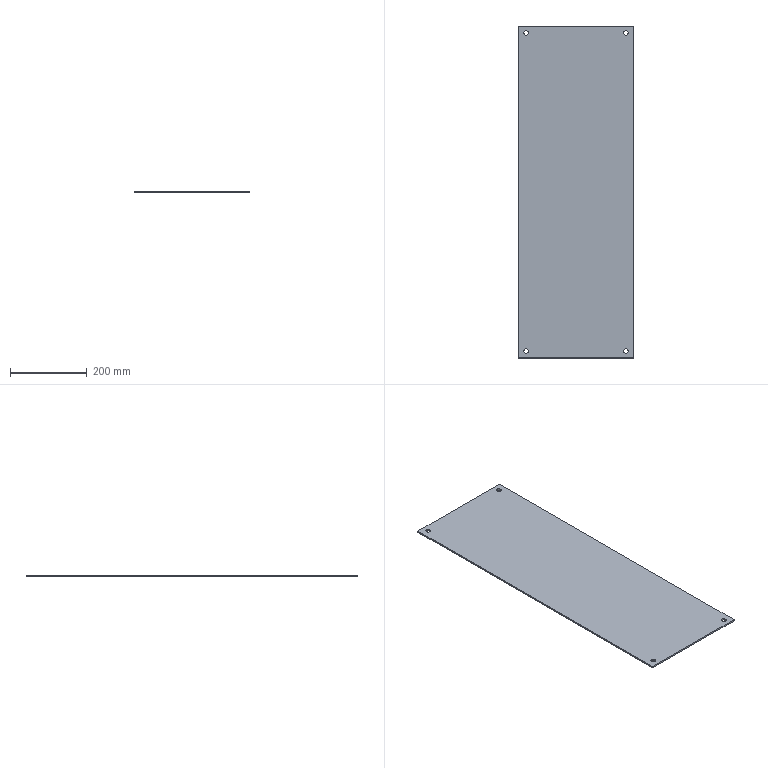Part | STEP file | 01 End cover plate | 1 solid | 14 faces | box 300 x 866 x 4 mm | volume 1037390 mm3 | cylinder 8 | plane 6 | commonest cylinder face diameters 12 x8
STEP:
#1=CARTESIAN_POINT('',(0.,0.,0.));
#2=DIRECTION('',(0.,0.,1.));
#3=DIRECTION('',(1.,0.,0.));
#4=AXIS2_PLACEMENT_3D('',#1,#2,#3);
#5=CARTESIAN_POINT('',(14.,-18.,4.));
#6=VERTEX_POINT('',#5);
#7=CARTESIAN_POINT('',(14.,-18.,0.));
#8=VERTEX_POINT('',#7);
#9=CARTESIAN_POINT('',(14.,-18.,4.));
#10=DIRECTION('',(0.,0.,-1.));
#11=VECTOR('',#10,1.);
#12=LINE('',#9,#11);
#13=CARTESIAN_POINT('',(20.,-18.,4.));
#14=DIRECTION('',(0.,0.,-1.));
#15=DIRECTION('',(-1.,0.,0.));
#16=AXIS2_PLACEMENT_3D('',#13,#14,#15);
#17=CYLINDRICAL_SURFACE('',#16,6.);
#18=CARTESIAN_POINT('',(6.283,0.));
#19=DIRECTION('',(0.,1.));
#20=VECTOR('',#19,1.);
#21=LINE('',#18,#20);
#22=(GEOMETRIC_REPRESENTATION_CONTEXT(2)PARAMETRIC_REPRESENTATION_CONTEXT()REPRESENTATION_CONTEXT('',''));
#23=DEFINITIONAL_REPRESENTATION('',(#21),#22);
#24=PCURVE('',#17,#23);
#25=CARTESIAN_POINT('',(20.,-18.,4.));
#26=DIRECTION('',(0.,0.,-1.));
#27=DIRECTION('',(-1.,0.,0.));
#28=AXIS2_PLACEMENT_3D('',#25,#26,#27);
#29=CYLINDRICAL_SURFACE('',#28,6.);
#30=CARTESIAN_POINT('',(0.,0.));
#31=DIRECTION('',(0.,1.));
#32=VECTOR('',#31,1.);
#33=LINE('',#30,#32);
#34=(GEOMETRIC_REPRESENTATION_CONTEXT(2)PARAMETRIC_REPRESENTATION_CONTEXT()REPRESENTATION_CONTEXT('',''));
#35=DEFINITIONAL_REPRESENTATION('',(#33),#34);
#36=PCURVE('',#29,#35);
#37=SURFACE_CURVE('',#12,(#24,#36),.PCURVE_S1.);
#38=EDGE_CURVE('',#6,#8,#37,.T.);
#39=ORIENTED_EDGE('',*,*,#38,.T.);
#40=CARTESIAN_POINT('',(26.,-18.,0.));
#41=VERTEX_POINT('',#40);
#42=CARTESIAN_POINT('',(20.,-18.,0.));
#43=DIRECTION('',(0.,0.,1.));
#44=DIRECTION('',(1.,0.,0.));
#45=AXIS2_PLACEMENT_3D('',#42,#43,#44);
#46=CIRCLE('',#45,6.);
#47=CARTESIAN_POINT('',(9.425,4.));
#48=DIRECTION('',(-1.,0.));
#49=VECTOR('',#48,1.);
#50=LINE('',#47,#49);
#51=(GEOMETRIC_REPRESENTATION_CONTEXT(2)PARAMETRIC_REPRESENTATION_CONTEXT()REPRESENTATION_CONTEXT('',''));
#52=DEFINITIONAL_REPRESENTATION('',(#50),#51);
#53=PCURVE('',#17,#52);
#54=CARTESIAN_POINT('',(0.,0.,0.));
#55=DIRECTION('',(0.,0.,1.));
#56=DIRECTION('',(1.,0.,0.));
#57=AXIS2_PLACEMENT_3D('',#54,#55,#56);
#58=PLANE('',#57);
#59=CARTESIAN_POINT('',(20.,-18.));
#60=DIRECTION('',(1.,0.));
#61=AXIS2_PLACEMENT_2D('',#59,#60);
#62=CIRCLE('',#61,6.);
#63=(GEOMETRIC_REPRESENTATION_CONTEXT(2)PARAMETRIC_REPRESENTATION_CONTEXT()REPRESENTATION_CONTEXT('',''));
#64=DEFINITIONAL_REPRESENTATION('',(#62),#63);
#65=PCURVE('',#58,#64);
#66=SURFACE_CURVE('',#46,(#53,#65),.PCURVE_S1.);
#67=EDGE_CURVE('',#8,#41,#66,.T.);
#68=ORIENTED_EDGE('',*,*,#67,.T.);
#69=CARTESIAN_POINT('',(26.,-18.,4.));
#70=VERTEX_POINT('',#69);
#71=CARTESIAN_POINT('',(26.,-18.,4.));
#72=DIRECTION('',(0.,0.,-1.));
#73=VECTOR('',#72,1.);
#74=LINE('',#71,#73);
#75=CARTESIAN_POINT('',(3.142,0.));
#76=DIRECTION('',(0.,1.));
#77=VECTOR('',#76,1.);
#78=LINE('',#75,#77);
#79=(GEOMETRIC_REPRESENTATION_CONTEXT(2)PARAMETRIC_REPRESENTATION_CONTEXT()REPRESENTATION_CONTEXT('',''));
#80=DEFINITIONAL_REPRESENTATION('',(#78),#79);
#81=PCURVE('',#17,#80);
#82=CARTESIAN_POINT('',(3.142,0.));
#83=DIRECTION('',(0.,1.));
#84=VECTOR('',#83,1.);
#85=LINE('',#82,#84);
#86=(GEOMETRIC_REPRESENTATION_CONTEXT(2)PARAMETRIC_REPRESENTATION_CONTEXT()REPRESENTATION_CONTEXT('',''));
#87=DEFINITIONAL_REPRESENTATION('',(#85),#86);
#88=PCURVE('',#29,#87);
#89=SURFACE_CURVE('',#74,(#81,#88),.PCURVE_S1.);
#90=EDGE_CURVE('',#70,#41,#89,.T.);
#91=ORIENTED_EDGE('',*,*,#90,.F.);
#92=CARTESIAN_POINT('',(20.,-18.,4.));
#93=DIRECTION('',(0.,0.,1.));
#94=DIRECTION('',(1.,0.,0.));
#95=AXIS2_PLACEMENT_3D('',#92,#93,#94);
#96=CIRCLE('',#95,6.);
#97=CARTESIAN_POINT('',(9.425,0.));
#98=DIRECTION('',(-1.,0.));
#99=VECTOR('',#98,1.);
#100=LINE('',#97,#99);
#101=(GEOMETRIC_REPRESENTATION_CONTEXT(2)PARAMETRIC_REPRESENTATION_CONTEXT()REPRESENTATION_CONTEXT('',''));
#102=DEFINITIONAL_REPRESENTATION('',(#100),#101);
#103=PCURVE('',#17,#102);
#104=CARTESIAN_POINT('',(0.,0.,4.));
#105=DIRECTION('',(0.,0.,1.));
#106=DIRECTION('',(1.,0.,0.));
#107=AXIS2_PLACEMENT_3D('',#104,#105,#106);
#108=PLANE('',#107);
#109=CARTESIAN_POINT('',(20.,-18.));
#110=DIRECTION('',(1.,0.));
#111=AXIS2_PLACEMENT_2D('',#109,#110);
#112=CIRCLE('',#111,6.);
#113=(GEOMETRIC_REPRESENTATION_CONTEXT(2)PARAMETRIC_REPRESENTATION_CONTEXT()REPRESENTATION_CONTEXT('',''));
#114=DEFINITIONAL_REPRESENTATION('',(#112),#113);
#115=PCURVE('',#108,#114);
#116=SURFACE_CURVE('',#96,(#103,#115),.PCURVE_S1.);
#117=EDGE_CURVE('',#6,#70,#116,.T.);
#118=ORIENTED_EDGE('',*,*,#117,.F.);
#119=EDGE_LOOP('',(#39,#68,#91,#118));
#120=FACE_BOUND('',#119,.F.);
#121=ADVANCED_FACE('',(#120),#17,.F.);
#122=CARTESIAN_POINT('',(274.,-18.,4.));
#123=VERTEX_POINT('',#122);
#124=CARTESIAN_POINT('',(274.,-18.,0.));
#125=VERTEX_POINT('',#124);
#126=CARTESIAN_POINT('',(274.,-18.,4.));
#127=DIRECTION('',(0.,0.,-1.));
#128=VECTOR('',#127,1.);
#129=LINE('',#126,#128);
#130=CARTESIAN_POINT('',(280.,-18.,4.));
#131=DIRECTION('',(0.,0.,-1.));
#132=DIRECTION('',(-1.,0.,0.));
#133=AXIS2_PLACEMENT_3D('',#130,#131,#132);
#134=CYLINDRICAL_SURFACE('',#133,6.);
#135=CARTESIAN_POINT('',(6.283,0.));
#136=DIRECTION('',(0.,1.));
#137=VECTOR('',#136,1.);
#138=LINE('',#135,#137);
#139=(GEOMETRIC_REPRESENTATION_CONTEXT(2)PARAMETRIC_REPRESENTATION_CONTEXT()REPRESENTATION_CONTEXT('',''));
#140=DEFINITIONAL_REPRESENTATION('',(#138),#139);
#141=PCURVE('',#134,#140);
#142=CARTESIAN_POINT('',(280.,-18.,4.));
#143=DIRECTION('',(0.,0.,-1.));
#144=DIRECTION('',(-1.,0.,0.));
#145=AXIS2_PLACEMENT_3D('',#142,#143,#144);
#146=CYLINDRICAL_SURFACE('',#145,6.);
#147=CARTESIAN_POINT('',(0.,0.));
#148=DIRECTION('',(0.,1.));
#149=VECTOR('',#148,1.);
#150=LINE('',#147,#149);
#151=(GEOMETRIC_REPRESENTATION_CONTEXT(2)PARAMETRIC_REPRESENTATION_CONTEXT()REPRESENTATION_CONTEXT('',''));
#152=DEFINITIONAL_REPRESENTATION('',(#150),#151);
#153=PCURVE('',#146,#152);
#154=SURFACE_CURVE('',#129,(#141,#153),.PCURVE_S1.);
#155=EDGE_CURVE('',#123,#125,#154,.T.);
#156=ORIENTED_EDGE('',*,*,#155,.T.);
#157=CARTESIAN_POINT('',(286.,-18.,0.));
#158=VERTEX_POINT('',#157);
#159=CARTESIAN_POINT('',(280.,-18.,0.));
#160=DIRECTION('',(0.,0.,1.));
#161=DIRECTION('',(1.,0.,0.));
#162=AXIS2_PLACEMENT_3D('',#159,#160,#161);
#163=CIRCLE('',#162,6.);
#164=CARTESIAN_POINT('',(9.425,4.));
#165=DIRECTION('',(-1.,0.));
#166=VECTOR('',#165,1.);
#167=LINE('',#164,#166);
#168=(GEOMETRIC_REPRESENTATION_CONTEXT(2)PARAMETRIC_REPRESENTATION_CONTEXT()REPRESENTATION_CONTEXT('',''));
#169=DEFINITIONAL_REPRESENTATION('',(#167),#168);
#170=PCURVE('',#134,#169);
#171=CARTESIAN_POINT('',(280.,-18.));
#172=DIRECTION('',(1.,0.));
#173=AXIS2_PLACEMENT_2D('',#171,#172);
#174=CIRCLE('',#173,6.);
#175=(GEOMETRIC_REPRESENTATION_CONTEXT(2)PARAMETRIC_REPRESENTATION_CONTEXT()REPRESENTATION_CONTEXT('',''));
#176=DEFINITIONAL_REPRESENTATION('',(#174),#175);
#177=PCURVE('',#58,#176);
#178=SURFACE_CURVE('',#163,(#170,#177),.PCURVE_S1.);
#179=EDGE_CURVE('',#125,#158,#178,.T.);
#180=ORIENTED_EDGE('',*,*,#179,.T.);
#181=CARTESIAN_POINT('',(286.,-18.,4.));
#182=VERTEX_POINT('',#181);
#183=CARTESIAN_POINT('',(286.,-18.,4.));
#184=DIRECTION('',(0.,0.,-1.));
#185=VECTOR('',#184,1.);
#186=LINE('',#183,#185);
#187=CARTESIAN_POINT('',(3.142,0.));
#188=DIRECTION('',(0.,1.));
#189=VECTOR('',#188,1.);
#190=LINE('',#187,#189);
#191=(GEOMETRIC_REPRESENTATION_CONTEXT(2)PARAMETRIC_REPRESENTATION_CONTEXT()REPRESENTATION_CONTEXT('',''));
#192=DEFINITIONAL_REPRESENTATION('',(#190),#191);
#193=PCURVE('',#134,#192);
#194=CARTESIAN_POINT('',(3.142,0.));
#195=DIRECTION('',(0.,1.));
#196=VECTOR('',#195,1.);
#197=LINE('',#194,#196);
#198=(GEOMETRIC_REPRESENTATION_CONTEXT(2)PARAMETRIC_REPRESENTATION_CONTEXT()REPRESENTATION_CONTEXT('',''));
#199=DEFINITIONAL_REPRESENTATION('',(#197),#198);
#200=PCURVE('',#146,#199);
#201=SURFACE_CURVE('',#186,(#193,#200),.PCURVE_S1.);
#202=EDGE_CURVE('',#182,#158,#201,.T.);
#203=ORIENTED_EDGE('',*,*,#202,.F.);
#204=CARTESIAN_POINT('',(280.,-18.,4.));
#205=DIRECTION('',(0.,0.,1.));
#206=DIRECTION('',(1.,0.,0.));
#207=AXIS2_PLACEMENT_3D('',#204,#205,#206);
#208=CIRCLE('',#207,6.);
#209=CARTESIAN_POINT('',(9.425,0.));
#210=DIRECTION('',(-1.,0.));
#211=VECTOR('',#210,1.);
#212=LINE('',#209,#211);
#213=(GEOMETRIC_REPRESENTATION_CONTEXT(2)PARAMETRIC_REPRESENTATION_CONTEXT()REPRESENTATION_CONTEXT('',''));
#214=DEFINITIONAL_REPRESENTATION('',(#212),#213);
#215=PCURVE('',#134,#214);
#216=CARTESIAN_POINT('',(280.,-18.));
#217=DIRECTION('',(1.,0.));
#218=AXIS2_PLACEMENT_2D('',#216,#217);
#219=CIRCLE('',#218,6.);
#220=(GEOMETRIC_REPRESENTATION_CONTEXT(2)PARAMETRIC_REPRESENTATION_CONTEXT()REPRESENTATION_CONTEXT('',''));
#221=DEFINITIONAL_REPRESENTATION('',(#219),#220);
#222=PCURVE('',#108,#221);
#223=SURFACE_CURVE('',#208,(#215,#222),.PCURVE_S1.);
#224=EDGE_CURVE('',#123,#182,#223,.T.);
#225=ORIENTED_EDGE('',*,*,#224,.F.);
#226=EDGE_LOOP('',(#156,#180,#203,#225));
#227=FACE_BOUND('',#226,.F.);
#228=ADVANCED_FACE('',(#227),#134,.F.);
#229=CARTESIAN_POINT('',(274.,-848.,4.));
#230=VERTEX_POINT('',#229);
#231=CARTESIAN_POINT('',(274.,-848.,0.));
#232=VERTEX_POINT('',#231);
#233=CARTESIAN_POINT('',(274.,-848.,4.));
#234=DIRECTION('',(0.,0.,-1.));
#235=VECTOR('',#234,1.);
#236=LINE('',#233,#235);
#237=CARTESIAN_POINT('',(280.,-848.,4.));
#238=DIRECTION('',(0.,0.,-1.));
#239=DIRECTION('',(-1.,0.,0.));
#240=AXIS2_PLACEMENT_3D('',#237,#238,#239);
#241=CYLINDRICAL_SURFACE('',#240,6.);
#242=CARTESIAN_POINT('',(6.283,0.));
#243=DIRECTION('',(0.,1.));
#244=VECTOR('',#243,1.);
#245=LINE('',#242,#244);
#246=(GEOMETRIC_REPRESENTATION_CONTEXT(2)PARAMETRIC_REPRESENTATION_CONTEXT()REPRESENTATION_CONTEXT('',''));
#247=DEFINITIONAL_REPRESENTATION('',(#245),#246);
#248=PCURVE('',#241,#247);
#249=CARTESIAN_POINT('',(280.,-848.,4.));
#250=DIRECTION('',(0.,0.,-1.));
#251=DIRECTION('',(-1.,0.,0.));
#252=AXIS2_PLACEMENT_3D('',#249,#250,#251);
#253=CYLINDRICAL_SURFACE('',#252,6.);
#254=CARTESIAN_POINT('',(0.,0.));
#255=DIRECTION('',(0.,1.));
#256=VECTOR('',#255,1.);
#257=LINE('',#254,#256);
#258=(GEOMETRIC_REPRESENTATION_CONTEXT(2)PARAMETRIC_REPRESENTATION_CONTEXT()REPRESENTATION_CONTEXT('',''));
#259=DEFINITIONAL_REPRESENTATION('',(#257),#258);
#260=PCURVE('',#253,#259);
#261=SURFACE_CURVE('',#236,(#248,#260),.PCURVE_S1.);
#262=EDGE_CURVE('',#230,#232,#261,.T.);
#263=ORIENTED_EDGE('',*,*,#262,.T.);
#264=CARTESIAN_POINT('',(286.,-848.,0.));
#265=VERTEX_POINT('',#264);
#266=CARTESIAN_POINT('',(280.,-848.,0.));
#267=DIRECTION('',(0.,0.,1.));
#268=DIRECTION('',(1.,0.,0.));
#269=AXIS2_PLACEMENT_3D('',#266,#267,#268);
#270=CIRCLE('',#269,6.);
#271=CARTESIAN_POINT('',(9.425,4.));
#272=DIRECTION('',(-1.,0.));
#273=VECTOR('',#272,1.);
#274=LINE('',#271,#273);
#275=(GEOMETRIC_REPRESENTATION_CONTEXT(2)PARAMETRIC_REPRESENTATION_CONTEXT()REPRESENTATION_CONTEXT('',''));
#276=DEFINITIONAL_REPRESENTATION('',(#274),#275);
#277=PCURVE('',#241,#276);
#278=CARTESIAN_POINT('',(280.,-848.));
#279=DIRECTION('',(1.,0.));
#280=AXIS2_PLACEMENT_2D('',#278,#279);
#281=CIRCLE('',#280,6.);
#282=(GEOMETRIC_REPRESENTATION_CONTEXT(2)PARAMETRIC_REPRESENTATION_CONTEXT()REPRESENTATION_CONTEXT('',''));
#283=DEFINITIONAL_REPRESENTATION('',(#281),#282);
#284=PCURVE('',#58,#283);
#285=SURFACE_CURVE('',#270,(#277,#284),.PCURVE_S1.);
#286=EDGE_CURVE('',#232,#265,#285,.T.);
#287=ORIENTED_EDGE('',*,*,#286,.T.);
#288=CARTESIAN_POINT('',(286.,-848.,4.));
#289=VERTEX_POINT('',#288);
#290=CARTESIAN_POINT('',(286.,-848.,4.));
#291=DIRECTION('',(0.,0.,-1.));
#292=VECTOR('',#291,1.);
#293=LINE('',#290,#292);
#294=CARTESIAN_POINT('',(3.142,0.));
#295=DIRECTION('',(0.,1.));
#296=VECTOR('',#295,1.);
#297=LINE('',#294,#296);
#298=(GEOMETRIC_REPRESENTATION_CONTEXT(2)PARAMETRIC_REPRESENTATION_CONTEXT()REPRESENTATION_CONTEXT('',''));
#299=DEFINITIONAL_REPRESENTATION('',(#297),#298);
#300=PCURVE('',#241,#299);
#301=CARTESIAN_POINT('',(3.142,0.));
#302=DIRECTION('',(0.,1.));
#303=VECTOR('',#302,1.);
#304=LINE('',#301,#303);
#305=(GEOMETRIC_REPRESENTATION_CONTEXT(2)PARAMETRIC_REPRESENTATION_CONTEXT()REPRESENTATION_CONTEXT('',''));
#306=DEFINITIONAL_REPRESENTATION('',(#304),#305);
#307=PCURVE('',#253,#306);
#308=SURFACE_CURVE('',#293,(#300,#307),.PCURVE_S1.);
#309=EDGE_CURVE('',#289,#265,#308,.T.);
#310=ORIENTED_EDGE('',*,*,#309,.F.);
#311=CARTESIAN_POINT('',(280.,-848.,4.));
#312=DIRECTION('',(0.,0.,1.));
#313=DIRECTION('',(1.,0.,0.));
#314=AXIS2_PLACEMENT_3D('',#311,#312,#313);
#315=CIRCLE('',#314,6.);
#316=CARTESIAN_POINT('',(9.425,0.));
#317=DIRECTION('',(-1.,0.));
#318=VECTOR('',#317,1.);
#319=LINE('',#316,#318);
#320=(GEOMETRIC_REPRESENTATION_CONTEXT(2)PARAMETRIC_REPRESENTATION_CONTEXT()REPRESENTATION_CONTEXT('',''));
#321=DEFINITIONAL_REPRESENTATION('',(#319),#320);
#322=PCURVE('',#241,#321);
#323=CARTESIAN_POINT('',(280.,-848.));
#324=DIRECTION('',(1.,0.));
#325=AXIS2_PLACEMENT_2D('',#323,#324);
#326=CIRCLE('',#325,6.);
#327=(GEOMETRIC_REPRESENTATION_CONTEXT(2)PARAMETRIC_REPRESENTATION_CONTEXT()REPRESENTATION_CONTEXT('',''));
#328=DEFINITIONAL_REPRESENTATION('',(#326),#327);
#329=PCURVE('',#108,#328);
#330=SURFACE_CURVE('',#315,(#322,#329),.PCURVE_S1.);
#331=EDGE_CURVE('',#230,#289,#330,.T.);
#332=ORIENTED_EDGE('',*,*,#331,.F.);
#333=EDGE_LOOP('',(#263,#287,#310,#332));
#334=FACE_BOUND('',#333,.F.);
#335=ADVANCED_FACE('',(#334),#241,.F.);
#336=CARTESIAN_POINT('',(14.,-848.,4.));
#337=VERTEX_POINT('',#336);
#338=CARTESIAN_POINT('',(14.,-848.,0.));
#339=VERTEX_POINT('',#338);
#340=CARTESIAN_POINT('',(14.,-848.,4.));
#341=DIRECTION('',(0.,0.,-1.));
#342=VECTOR('',#341,1.);
#343=LINE('',#340,#342);
#344=CARTESIAN_POINT('',(20.,-848.,4.));
#345=DIRECTION('',(0.,0.,-1.));
#346=DIRECTION('',(-1.,0.,0.));
#347=AXIS2_PLACEMENT_3D('',#344,#345,#346);
#348=CYLINDRICAL_SURFACE('',#347,6.);
#349=CARTESIAN_POINT('',(6.283,0.));
#350=DIRECTION('',(0.,1.));
#351=VECTOR('',#350,1.);
#352=LINE('',#349,#351);
#353=(GEOMETRIC_REPRESENTATION_CONTEXT(2)PARAMETRIC_REPRESENTATION_CONTEXT()REPRESENTATION_CONTEXT('',''));
#354=DEFINITIONAL_REPRESENTATION('',(#352),#353);
#355=PCURVE('',#348,#354);
#356=CARTESIAN_POINT('',(20.,-848.,4.));
#357=DIRECTION('',(0.,0.,-1.));
#358=DIRECTION('',(-1.,0.,0.));
#359=AXIS2_PLACEMENT_3D('',#356,#357,#358);
#360=CYLINDRICAL_SURFACE('',#359,6.);
#361=CARTESIAN_POINT('',(0.,0.));
#362=DIRECTION('',(0.,1.));
#363=VECTOR('',#362,1.);
#364=LINE('',#361,#363);
#365=(GEOMETRIC_REPRESENTATION_CONTEXT(2)PARAMETRIC_REPRESENTATION_CONTEXT()REPRESENTATION_CONTEXT('',''));
#366=DEFINITIONAL_REPRESENTATION('',(#364),#365);
#367=PCURVE('',#360,#366);
#368=SURFACE_CURVE('',#343,(#355,#367),.PCURVE_S1.);
#369=EDGE_CURVE('',#337,#339,#368,.T.);
#370=ORIENTED_EDGE('',*,*,#369,.T.);
#371=CARTESIAN_POINT('',(26.,-848.,0.));
#372=VERTEX_POINT('',#371);
#373=CARTESIAN_POINT('',(20.,-848.,0.));
#374=DIRECTION('',(0.,0.,1.));
#375=DIRECTION('',(1.,0.,0.));
#376=AXIS2_PLACEMENT_3D('',#373,#374,#375);
#377=CIRCLE('',#376,6.);
#378=CARTESIAN_POINT('',(9.425,4.));
#379=DIRECTION('',(-1.,0.));
#380=VECTOR('',#379,1.);
#381=LINE('',#378,#380);
#382=(GEOMETRIC_REPRESENTATION_CONTEXT(2)PARAMETRIC_REPRESENTATION_CONTEXT()REPRESENTATION_CONTEXT('',''));
#383=DEFINITIONAL_REPRESENTATION('',(#381),#382);
#384=PCURVE('',#348,#383);
#385=CARTESIAN_POINT('',(20.,-848.));
#386=DIRECTION('',(1.,0.));
#387=AXIS2_PLACEMENT_2D('',#385,#386);
#388=CIRCLE('',#387,6.);
#389=(GEOMETRIC_REPRESENTATION_CONTEXT(2)PARAMETRIC_REPRESENTATION_CONTEXT()REPRESENTATION_CONTEXT('',''));
#390=DEFINITIONAL_REPRESENTATION('',(#388),#389);
#391=PCURVE('',#58,#390);
#392=SURFACE_CURVE('',#377,(#384,#391),.PCURVE_S1.);
#393=EDGE_CURVE('',#339,#372,#392,.T.);
#394=ORIENTED_EDGE('',*,*,#393,.T.);
#395=CARTESIAN_POINT('',(26.,-848.,4.));
#396=VERTEX_POINT('',#395);
#397=CARTESIAN_POINT('',(26.,-848.,4.));
#398=DIRECTION('',(0.,0.,-1.));
#399=VECTOR('',#398,1.);
#400=LINE('',#397,#399);
#401=CARTESIAN_POINT('',(3.142,0.));
#402=DIRECTION('',(0.,1.));
#403=VECTOR('',#402,1.);
#404=LINE('',#401,#403);
#405=(GEOMETRIC_REPRESENTATION_CONTEXT(2)PARAMETRIC_REPRESENTATION_CONTEXT()REPRESENTATION_CONTEXT('',''));
#406=DEFINITIONAL_REPRESENTATION('',(#404),#405);
#407=PCURVE('',#348,#406);
#408=CARTESIAN_POINT('',(3.142,0.));
#409=DIRECTION('',(0.,1.));
#410=VECTOR('',#409,1.);
#411=LINE('',#408,#410);
#412=(GEOMETRIC_REPRESENTATION_CONTEXT(2)PARAMETRIC_REPRESENTATION_CONTEXT()REPRESENTATION_CONTEXT('',''));
#413=DEFINITIONAL_REPRESENTATION('',(#411),#412);
#414=PCURVE('',#360,#413);
#415=SURFACE_CURVE('',#400,(#407,#414),.PCURVE_S1.);
#416=EDGE_CURVE('',#396,#372,#415,.T.);
#417=ORIENTED_EDGE('',*,*,#416,.F.);
#418=CARTESIAN_POINT('',(20.,-848.,4.));
#419=DIRECTION('',(0.,0.,1.));
#420=DIRECTION('',(1.,0.,0.));
#421=AXIS2_PLACEMENT_3D('',#418,#419,#420);
#422=CIRCLE('',#421,6.);
#423=CARTESIAN_POINT('',(9.425,0.));
#424=DIRECTION('',(-1.,0.));
#425=VECTOR('',#424,1.);
#426=LINE('',#423,#425);
#427=(GEOMETRIC_REPRESENTATION_CONTEXT(2)PARAMETRIC_REPRESENTATION_CONTEXT()REPRESENTATION_CONTEXT('',''));
#428=DEFINITIONAL_REPRESENTATION('',(#426),#427);
#429=PCURVE('',#348,#428);
#430=CARTESIAN_POINT('',(20.,-848.));
#431=DIRECTION('',(1.,0.));
#432=AXIS2_PLACEMENT_2D('',#430,#431);
#433=CIRCLE('',#432,6.);
#434=(GEOMETRIC_REPRESENTATION_CONTEXT(2)PARAMETRIC_REPRESENTATION_CONTEXT()REPRESENTATION_CONTEXT('',''));
#435=DEFINITIONAL_REPRESENTATION('',(#433),#434);
#436=PCURVE('',#108,#435);
#437=SURFACE_CURVE('',#422,(#429,#436),.PCURVE_S1.);
#438=EDGE_CURVE('',#337,#396,#437,.T.);
#439=ORIENTED_EDGE('',*,*,#438,.F.);
#440=EDGE_LOOP('',(#370,#394,#417,#439));
#441=FACE_BOUND('',#440,.F.);
#442=ADVANCED_FACE('',(#441),#348,.F.);
#443=ORIENTED_EDGE('',*,*,#224,.F.);
#444=CARTESIAN_POINT('',(280.,-18.,4.));
#445=DIRECTION('',(0.,0.,1.));
#446=DIRECTION('',(1.,0.,0.));
#447=AXIS2_PLACEMENT_3D('',#444,#445,#446);
#448=CIRCLE('',#447,6.);
#449=CARTESIAN_POINT('',(280.,-18.));
#450=DIRECTION('',(1.,0.));
#451=AXIS2_PLACEMENT_2D('',#449,#450);
#452=CIRCLE('',#451,6.);
#453=(GEOMETRIC_REPRESENTATION_CONTEXT(2)PARAMETRIC_REPRESENTATION_CONTEXT()REPRESENTATION_CONTEXT('',''));
#454=DEFINITIONAL_REPRESENTATION('',(#452),#453);
#455=PCURVE('',#108,#454);
#456=CARTESIAN_POINT('',(3.142,0.));
#457=DIRECTION('',(-1.,0.));
#458=VECTOR('',#457,1.);
#459=LINE('',#456,#458);
#460=(GEOMETRIC_REPRESENTATION_CONTEXT(2)PARAMETRIC_REPRESENTATION_CONTEXT()REPRESENTATION_CONTEXT('',''));
#461=DEFINITIONAL_REPRESENTATION('',(#459),#460);
#462=PCURVE('',#146,#461);
#463=SURFACE_CURVE('',#448,(#455,#462),.PCURVE_S1.);
#464=EDGE_CURVE('',#182,#123,#463,.T.);
#465=ORIENTED_EDGE('',*,*,#464,.F.);
#466=EDGE_LOOP('',(#443,#465));
#467=FACE_BOUND('',#466,.T.);
#468=ORIENTED_EDGE('',*,*,#438,.F.);
#469=CARTESIAN_POINT('',(20.,-848.,4.));
#470=DIRECTION('',(0.,0.,1.));
#471=DIRECTION('',(1.,0.,0.));
#472=AXIS2_PLACEMENT_3D('',#469,#470,#471);
#473=CIRCLE('',#472,6.);
#474=CARTESIAN_POINT('',(20.,-848.));
#475=DIRECTION('',(1.,0.));
#476=AXIS2_PLACEMENT_2D('',#474,#475);
#477=CIRCLE('',#476,6.);
#478=(GEOMETRIC_REPRESENTATION_CONTEXT(2)PARAMETRIC_REPRESENTATION_CONTEXT()REPRESENTATION_CONTEXT('',''));
#479=DEFINITIONAL_REPRESENTATION('',(#477),#478);
#480=PCURVE('',#108,#479);
#481=CARTESIAN_POINT('',(3.142,0.));
#482=DIRECTION('',(-1.,0.));
#483=VECTOR('',#482,1.);
#484=LINE('',#481,#483);
#485=(GEOMETRIC_REPRESENTATION_CONTEXT(2)PARAMETRIC_REPRESENTATION_CONTEXT()REPRESENTATION_CONTEXT('',''));
#486=DEFINITIONAL_REPRESENTATION('',(#484),#485);
#487=PCURVE('',#360,#486);
#488=SURFACE_CURVE('',#473,(#480,#487),.PCURVE_S1.);
#489=EDGE_CURVE('',#396,#337,#488,.T.);
#490=ORIENTED_EDGE('',*,*,#489,.F.);
#491=EDGE_LOOP('',(#468,#490));
#492=FACE_BOUND('',#491,.T.);
#493=CARTESIAN_POINT('',(0.,0.,4.));
#494=VERTEX_POINT('',#493);
#495=CARTESIAN_POINT('',(0.,-866.,4.));
#496=VERTEX_POINT('',#495);
#497=CARTESIAN_POINT('',(0.,0.,4.));
#498=DIRECTION('',(0.,-1.,0.));
#499=VECTOR('',#498,1.);
#500=LINE('',#497,#499);
#501=CARTESIAN_POINT('',(0.,0.));
#502=DIRECTION('',(0.,-1.));
#503=VECTOR('',#502,1.);
#504=LINE('',#501,#503);
#505=(GEOMETRIC_REPRESENTATION_CONTEXT(2)PARAMETRIC_REPRESENTATION_CONTEXT()REPRESENTATION_CONTEXT('',''));
#506=DEFINITIONAL_REPRESENTATION('',(#504),#505);
#507=PCURVE('',#108,#506);
#508=CARTESIAN_POINT('',(0.,0.,4.));
#509=DIRECTION('',(1.,0.,0.));
#510=DIRECTION('',(0.,1.,0.));
#511=AXIS2_PLACEMENT_3D('',#508,#509,#510);
#512=PLANE('',#511);
#513=CARTESIAN_POINT('',(0.,0.));
#514=DIRECTION('',(-1.,0.));
#515=VECTOR('',#514,1.);
#516=LINE('',#513,#515);
#517=(GEOMETRIC_REPRESENTATION_CONTEXT(2)PARAMETRIC_REPRESENTATION_CONTEXT()REPRESENTATION_CONTEXT('',''));
#518=DEFINITIONAL_REPRESENTATION('',(#516),#517);
#519=PCURVE('',#512,#518);
#520=SURFACE_CURVE('',#500,(#507,#519),.PCURVE_S1.);
#521=EDGE_CURVE('',#494,#496,#520,.T.);
#522=ORIENTED_EDGE('',*,*,#521,.T.);
#523=CARTESIAN_POINT('',(300.,-866.,4.));
#524=VERTEX_POINT('',#523);
#525=CARTESIAN_POINT('',(0.,-866.,4.));
#526=DIRECTION('',(1.,0.,0.));
#527=VECTOR('',#526,1.);
#528=LINE('',#525,#527);
#529=CARTESIAN_POINT('',(0.,-866.));
#530=DIRECTION('',(1.,0.));
#531=VECTOR('',#530,1.);
#532=LINE('',#529,#531);
#533=(GEOMETRIC_REPRESENTATION_CONTEXT(2)PARAMETRIC_REPRESENTATION_CONTEXT()REPRESENTATION_CONTEXT('',''));
#534=DEFINITIONAL_REPRESENTATION('',(#532),#533);
#535=PCURVE('',#108,#534);
#536=CARTESIAN_POINT('',(0.,-866.,4.));
#537=DIRECTION('',(0.,1.,0.));
#538=DIRECTION('',(0.,0.,1.));
#539=AXIS2_PLACEMENT_3D('',#536,#537,#538);
#540=PLANE('',#539);
#541=CARTESIAN_POINT('',(0.,0.));
#542=DIRECTION('',(0.,1.));
#543=VECTOR('',#542,1.);
#544=LINE('',#541,#543);
#545=(GEOMETRIC_REPRESENTATION_CONTEXT(2)PARAMETRIC_REPRESENTATION_CONTEXT()REPRESENTATION_CONTEXT('',''));
#546=DEFINITIONAL_REPRESENTATION('',(#544),#545);
#547=PCURVE('',#540,#546);
#548=SURFACE_CURVE('',#528,(#535,#547),.PCURVE_S1.);
#549=EDGE_CURVE('',#496,#524,#548,.T.);
#550=ORIENTED_EDGE('',*,*,#549,.T.);
#551=CARTESIAN_POINT('',(300.,0.,4.));
#552=VERTEX_POINT('',#551);
#553=CARTESIAN_POINT('',(300.,0.,4.));
#554=DIRECTION('',(0.,1.,0.));
#555=VECTOR('',#554,1.);
#556=LINE('',#553,#555);
#557=CARTESIAN_POINT('',(300.,0.));
#558=DIRECTION('',(0.,1.));
#559=VECTOR('',#558,1.);
#560=LINE('',#557,#559);
#561=(GEOMETRIC_REPRESENTATION_CONTEXT(2)PARAMETRIC_REPRESENTATION_CONTEXT()REPRESENTATION_CONTEXT('',''));
#562=DEFINITIONAL_REPRESENTATION('',(#560),#561);
#563=PCURVE('',#108,#562);
#564=CARTESIAN_POINT('',(300.,0.,4.));
#565=DIRECTION('',(-1.,0.,0.));
#566=DIRECTION('',(0.,-1.,0.));
#567=AXIS2_PLACEMENT_3D('',#564,#565,#566);
#568=PLANE('',#567);
#569=CARTESIAN_POINT('',(0.,0.));
#570=DIRECTION('',(-1.,0.));
#571=VECTOR('',#570,1.);
#572=LINE('',#569,#571);
#573=(GEOMETRIC_REPRESENTATION_CONTEXT(2)PARAMETRIC_REPRESENTATION_CONTEXT()REPRESENTATION_CONTEXT('',''));
#574=DEFINITIONAL_REPRESENTATION('',(#572),#573);
#575=PCURVE('',#568,#574);
#576=SURFACE_CURVE('',#556,(#563,#575),.PCURVE_S1.);
#577=EDGE_CURVE('',#524,#552,#576,.T.);
#578=ORIENTED_EDGE('',*,*,#577,.T.);
#579=CARTESIAN_POINT('',(0.,0.,4.));
#580=DIRECTION('',(-1.,0.,0.));
#581=VECTOR('',#580,1.);
#582=LINE('',#579,#581);
#583=CARTESIAN_POINT('',(0.,0.));
#584=DIRECTION('',(-1.,0.));
#585=VECTOR('',#584,1.);
#586=LINE('',#583,#585);
#587=(GEOMETRIC_REPRESENTATION_CONTEXT(2)PARAMETRIC_REPRESENTATION_CONTEXT()REPRESENTATION_CONTEXT('',''));
#588=DEFINITIONAL_REPRESENTATION('',(#586),#587);
#589=PCURVE('',#108,#588);
#590=CARTESIAN_POINT('',(0.,0.,4.));
#591=DIRECTION('',(0.,-1.,0.));
#592=DIRECTION('',(0.,0.,-1.));
#593=AXIS2_PLACEMENT_3D('',#590,#591,#592);
#594=PLANE('',#593);
#595=CARTESIAN_POINT('',(0.,0.));
#596=DIRECTION('',(0.,-1.));
#597=VECTOR('',#596,1.);
#598=LINE('',#595,#597);
#599=(GEOMETRIC_REPRESENTATION_CONTEXT(2)PARAMETRIC_REPRESENTATION_CONTEXT()REPRESENTATION_CONTEXT('',''));
#600=DEFINITIONAL_REPRESENTATION('',(#598),#599);
#601=PCURVE('',#594,#600);
#602=SURFACE_CURVE('',#582,(#589,#601),.PCURVE_S1.);
#603=EDGE_CURVE('',#552,#494,#602,.T.);
#604=ORIENTED_EDGE('',*,*,#603,.T.);
#605=EDGE_LOOP('',(#522,#550,#578,#604));
#606=FACE_BOUND('',#605,.T.);
#607=ORIENTED_EDGE('',*,*,#331,.F.);
#608=CARTESIAN_POINT('',(280.,-848.,4.));
#609=DIRECTION('',(0.,0.,1.));
#610=DIRECTION('',(1.,0.,0.));
#611=AXIS2_PLACEMENT_3D('',#608,#609,#610);
#612=CIRCLE('',#611,6.);
#613=CARTESIAN_POINT('',(280.,-848.));
#614=DIRECTION('',(1.,0.));
#615=AXIS2_PLACEMENT_2D('',#613,#614);
#616=CIRCLE('',#615,6.);
#617=(GEOMETRIC_REPRESENTATION_CONTEXT(2)PARAMETRIC_REPRESENTATION_CONTEXT()REPRESENTATION_CONTEXT('',''));
#618=DEFINITIONAL_REPRESENTATION('',(#616),#617);
#619=PCURVE('',#108,#618);
#620=CARTESIAN_POINT('',(3.142,0.));
#621=DIRECTION('',(-1.,0.));
#622=VECTOR('',#621,1.);
#623=LINE('',#620,#622);
#624=(GEOMETRIC_REPRESENTATION_CONTEXT(2)PARAMETRIC_REPRESENTATION_CONTEXT()REPRESENTATION_CONTEXT('',''));
#625=DEFINITIONAL_REPRESENTATION('',(#623),#624);
#626=PCURVE('',#253,#625);
#627=SURFACE_CURVE('',#612,(#619,#626),.PCURVE_S1.);
#628=EDGE_CURVE('',#289,#230,#627,.T.);
#629=ORIENTED_EDGE('',*,*,#628,.F.);
#630=EDGE_LOOP('',(#607,#629));
#631=FACE_BOUND('',#630,.T.);
#632=ORIENTED_EDGE('',*,*,#117,.F.);
#633=CARTESIAN_POINT('',(20.,-18.,4.));
#634=DIRECTION('',(0.,0.,1.));
#635=DIRECTION('',(1.,0.,0.));
#636=AXIS2_PLACEMENT_3D('',#633,#634,#635);
#637=CIRCLE('',#636,6.);
#638=CARTESIAN_POINT('',(20.,-18.));
#639=DIRECTION('',(1.,0.));
#640=AXIS2_PLACEMENT_2D('',#638,#639);
#641=CIRCLE('',#640,6.);
#642=(GEOMETRIC_REPRESENTATION_CONTEXT(2)PARAMETRIC_REPRESENTATION_CONTEXT()REPRESENTATION_CONTEXT('',''));
#643=DEFINITIONAL_REPRESENTATION('',(#641),#642);
#644=PCURVE('',#108,#643);
#645=CARTESIAN_POINT('',(3.142,0.));
#646=DIRECTION('',(-1.,0.));
#647=VECTOR('',#646,1.);
#648=LINE('',#645,#647);
#649=(GEOMETRIC_REPRESENTATION_CONTEXT(2)PARAMETRIC_REPRESENTATION_CONTEXT()REPRESENTATION_CONTEXT('',''));
#650=DEFINITIONAL_REPRESENTATION('',(#648),#649);
#651=PCURVE('',#29,#650);
#652=SURFACE_CURVE('',#637,(#644,#651),.PCURVE_S1.);
#653=EDGE_CURVE('',#70,#6,#652,.T.);
#654=ORIENTED_EDGE('',*,*,#653,.F.);
#655=EDGE_LOOP('',(#632,#654));
#656=FACE_BOUND('',#655,.T.);
#657=ADVANCED_FACE('',(#467,#492,#606,#631,#656),#108,.T.);
#658=ORIENTED_EDGE('',*,*,#179,.T.);
#659=CARTESIAN_POINT('',(280.,-18.,0.));
#660=DIRECTION('',(0.,0.,1.));
#661=DIRECTION('',(1.,0.,0.));
#662=AXIS2_PLACEMENT_3D('',#659,#660,#661);
#663=CIRCLE('',#662,6.);
#664=CARTESIAN_POINT('',(280.,-18.));
#665=DIRECTION('',(1.,0.));
#666=AXIS2_PLACEMENT_2D('',#664,#665);
#667=CIRCLE('',#666,6.);
#668=(GEOMETRIC_REPRESENTATION_CONTEXT(2)PARAMETRIC_REPRESENTATION_CONTEXT()REPRESENTATION_CONTEXT('',''));
#669=DEFINITIONAL_REPRESENTATION('',(#667),#668);
#670=PCURVE('',#58,#669);
#671=CARTESIAN_POINT('',(3.142,4.));
#672=DIRECTION('',(-1.,0.));
#673=VECTOR('',#672,1.);
#674=LINE('',#671,#673);
#675=(GEOMETRIC_REPRESENTATION_CONTEXT(2)PARAMETRIC_REPRESENTATION_CONTEXT()REPRESENTATION_CONTEXT('',''));
#676=DEFINITIONAL_REPRESENTATION('',(#674),#675);
#677=PCURVE('',#146,#676);
#678=SURFACE_CURVE('',#663,(#670,#677),.PCURVE_S1.);
#679=EDGE_CURVE('',#158,#125,#678,.T.);
#680=ORIENTED_EDGE('',*,*,#679,.T.);
#681=EDGE_LOOP('',(#658,#680));
#682=FACE_BOUND('',#681,.T.);
#683=ORIENTED_EDGE('',*,*,#393,.T.);
#684=CARTESIAN_POINT('',(20.,-848.,0.));
#685=DIRECTION('',(0.,0.,1.));
#686=DIRECTION('',(1.,0.,0.));
#687=AXIS2_PLACEMENT_3D('',#684,#685,#686);
#688=CIRCLE('',#687,6.);
#689=CARTESIAN_POINT('',(20.,-848.));
#690=DIRECTION('',(1.,0.));
#691=AXIS2_PLACEMENT_2D('',#689,#690);
#692=CIRCLE('',#691,6.);
#693=(GEOMETRIC_REPRESENTATION_CONTEXT(2)PARAMETRIC_REPRESENTATION_CONTEXT()REPRESENTATION_CONTEXT('',''));
#694=DEFINITIONAL_REPRESENTATION('',(#692),#693);
#695=PCURVE('',#58,#694);
#696=CARTESIAN_POINT('',(3.142,4.));
#697=DIRECTION('',(-1.,0.));
#698=VECTOR('',#697,1.);
#699=LINE('',#696,#698);
#700=(GEOMETRIC_REPRESENTATION_CONTEXT(2)PARAMETRIC_REPRESENTATION_CONTEXT()REPRESENTATION_CONTEXT('',''));
#701=DEFINITIONAL_REPRESENTATION('',(#699),#700);
#702=PCURVE('',#360,#701);
#703=SURFACE_CURVE('',#688,(#695,#702),.PCURVE_S1.);
#704=EDGE_CURVE('',#372,#339,#703,.T.);
#705=ORIENTED_EDGE('',*,*,#704,.T.);
#706=EDGE_LOOP('',(#683,#705));
#707=FACE_BOUND('',#706,.T.);
#708=CARTESIAN_POINT('',(0.,0.,0.));
#709=VERTEX_POINT('',#708);
#710=CARTESIAN_POINT('',(0.,-866.,0.));
#711=VERTEX_POINT('',#710);
#712=CARTESIAN_POINT('',(0.,0.,0.));
#713=DIRECTION('',(0.,-1.,0.));
#714=VECTOR('',#713,1.);
#715=LINE('',#712,#714);
#716=CARTESIAN_POINT('',(0.,0.));
#717=DIRECTION('',(0.,-1.));
#718=VECTOR('',#717,1.);
#719=LINE('',#716,#718);
#720=(GEOMETRIC_REPRESENTATION_CONTEXT(2)PARAMETRIC_REPRESENTATION_CONTEXT()REPRESENTATION_CONTEXT('',''));
#721=DEFINITIONAL_REPRESENTATION('',(#719),#720);
#722=PCURVE('',#58,#721);
#723=CARTESIAN_POINT('',(0.,-4.));
#724=DIRECTION('',(-1.,0.));
#725=VECTOR('',#724,1.);
#726=LINE('',#723,#725);
#727=(GEOMETRIC_REPRESENTATION_CONTEXT(2)PARAMETRIC_REPRESENTATION_CONTEXT()REPRESENTATION_CONTEXT('',''));
#728=DEFINITIONAL_REPRESENTATION('',(#726),#727);
#729=PCURVE('',#512,#728);
#730=SURFACE_CURVE('',#715,(#722,#729),.PCURVE_S1.);
#731=EDGE_CURVE('',#709,#711,#730,.T.);
#732=ORIENTED_EDGE('',*,*,#731,.F.);
#733=CARTESIAN_POINT('',(300.,0.,0.));
#734=VERTEX_POINT('',#733);
#735=CARTESIAN_POINT('',(0.,0.,0.));
#736=DIRECTION('',(-1.,0.,0.));
#737=VECTOR('',#736,1.);
#738=LINE('',#735,#737);
#739=CARTESIAN_POINT('',(0.,0.));
#740=DIRECTION('',(-1.,0.));
#741=VECTOR('',#740,1.);
#742=LINE('',#739,#741);
#743=(GEOMETRIC_REPRESENTATION_CONTEXT(2)PARAMETRIC_REPRESENTATION_CONTEXT()REPRESENTATION_CONTEXT('',''));
#744=DEFINITIONAL_REPRESENTATION('',(#742),#743);
#745=PCURVE('',#58,#744);
#746=CARTESIAN_POINT('',(4.,0.));
#747=DIRECTION('',(0.,-1.));
#748=VECTOR('',#747,1.);
#749=LINE('',#746,#748);
#750=(GEOMETRIC_REPRESENTATION_CONTEXT(2)PARAMETRIC_REPRESENTATION_CONTEXT()REPRESENTATION_CONTEXT('',''));
#751=DEFINITIONAL_REPRESENTATION('',(#749),#750);
#752=PCURVE('',#594,#751);
#753=SURFACE_CURVE('',#738,(#745,#752),.PCURVE_S1.);
#754=EDGE_CURVE('',#734,#709,#753,.T.);
#755=ORIENTED_EDGE('',*,*,#754,.F.);
#756=CARTESIAN_POINT('',(300.,-866.,0.));
#757=VERTEX_POINT('',#756);
#758=CARTESIAN_POINT('',(300.,0.,0.));
#759=DIRECTION('',(0.,1.,0.));
#760=VECTOR('',#759,1.);
#761=LINE('',#758,#760);
#762=CARTESIAN_POINT('',(300.,0.));
#763=DIRECTION('',(0.,1.));
#764=VECTOR('',#763,1.);
#765=LINE('',#762,#764);
#766=(GEOMETRIC_REPRESENTATION_CONTEXT(2)PARAMETRIC_REPRESENTATION_CONTEXT()REPRESENTATION_CONTEXT('',''));
#767=DEFINITIONAL_REPRESENTATION('',(#765),#766);
#768=PCURVE('',#58,#767);
#769=CARTESIAN_POINT('',(0.,-4.));
#770=DIRECTION('',(-1.,0.));
#771=VECTOR('',#770,1.);
#772=LINE('',#769,#771);
#773=(GEOMETRIC_REPRESENTATION_CONTEXT(2)PARAMETRIC_REPRESENTATION_CONTEXT()REPRESENTATION_CONTEXT('',''));
#774=DEFINITIONAL_REPRESENTATION('',(#772),#773);
#775=PCURVE('',#568,#774);
#776=SURFACE_CURVE('',#761,(#768,#775),.PCURVE_S1.);
#777=EDGE_CURVE('',#757,#734,#776,.T.);
#778=ORIENTED_EDGE('',*,*,#777,.F.);
#779=CARTESIAN_POINT('',(0.,-866.,0.));
#780=DIRECTION('',(1.,0.,0.));
#781=VECTOR('',#780,1.);
#782=LINE('',#779,#781);
#783=CARTESIAN_POINT('',(0.,-866.));
#784=DIRECTION('',(1.,0.));
#785=VECTOR('',#784,1.);
#786=LINE('',#783,#785);
#787=(GEOMETRIC_REPRESENTATION_CONTEXT(2)PARAMETRIC_REPRESENTATION_CONTEXT()REPRESENTATION_CONTEXT('',''));
#788=DEFINITIONAL_REPRESENTATION('',(#786),#787);
#789=PCURVE('',#58,#788);
#790=CARTESIAN_POINT('',(-4.,0.));
#791=DIRECTION('',(0.,1.));
#792=VECTOR('',#791,1.);
#793=LINE('',#790,#792);
#794=(GEOMETRIC_REPRESENTATION_CONTEXT(2)PARAMETRIC_REPRESENTATION_CONTEXT()REPRESENTATION_CONTEXT('',''));
#795=DEFINITIONAL_REPRESENTATION('',(#793),#794);
#796=PCURVE('',#540,#795);
#797=SURFACE_CURVE('',#782,(#789,#796),.PCURVE_S1.);
#798=EDGE_CURVE('',#711,#757,#797,.T.);
#799=ORIENTED_EDGE('',*,*,#798,.F.);
#800=EDGE_LOOP('',(#732,#755,#778,#799));
#801=FACE_BOUND('',#800,.T.);
#802=ORIENTED_EDGE('',*,*,#286,.T.);
#803=CARTESIAN_POINT('',(280.,-848.,0.));
#804=DIRECTION('',(0.,0.,1.));
#805=DIRECTION('',(1.,0.,0.));
#806=AXIS2_PLACEMENT_3D('',#803,#804,#805);
#807=CIRCLE('',#806,6.);
#808=CARTESIAN_POINT('',(280.,-848.));
#809=DIRECTION('',(1.,0.));
#810=AXIS2_PLACEMENT_2D('',#808,#809);
#811=CIRCLE('',#810,6.);
#812=(GEOMETRIC_REPRESENTATION_CONTEXT(2)PARAMETRIC_REPRESENTATION_CONTEXT()REPRESENTATION_CONTEXT('',''));
#813=DEFINITIONAL_REPRESENTATION('',(#811),#812);
#814=PCURVE('',#58,#813);
#815=CARTESIAN_POINT('',(3.142,4.));
#816=DIRECTION('',(-1.,0.));
#817=VECTOR('',#816,1.);
#818=LINE('',#815,#817);
#819=(GEOMETRIC_REPRESENTATION_CONTEXT(2)PARAMETRIC_REPRESENTATION_CONTEXT()REPRESENTATION_CONTEXT('',''));
#820=DEFINITIONAL_REPRESENTATION('',(#818),#819);
#821=PCURVE('',#253,#820);
#822=SURFACE_CURVE('',#807,(#814,#821),.PCURVE_S1.);
#823=EDGE_CURVE('',#265,#232,#822,.T.);
#824=ORIENTED_EDGE('',*,*,#823,.T.);
#825=EDGE_LOOP('',(#802,#824));
#826=FACE_BOUND('',#825,.T.);
#827=ORIENTED_EDGE('',*,*,#67,.T.);
#828=CARTESIAN_POINT('',(20.,-18.,0.));
#829=DIRECTION('',(0.,0.,1.));
#830=DIRECTION('',(1.,0.,0.));
#831=AXIS2_PLACEMENT_3D('',#828,#829,#830);
#832=CIRCLE('',#831,6.);
#833=CARTESIAN_POINT('',(20.,-18.));
#834=DIRECTION('',(1.,0.));
#835=AXIS2_PLACEMENT_2D('',#833,#834);
#836=CIRCLE('',#835,6.);
#837=(GEOMETRIC_REPRESENTATION_CONTEXT(2)PARAMETRIC_REPRESENTATION_CONTEXT()REPRESENTATION_CONTEXT('',''));
#838=DEFINITIONAL_REPRESENTATION('',(#836),#837);
#839=PCURVE('',#58,#838);
#840=CARTESIAN_POINT('',(3.142,4.));
#841=DIRECTION('',(-1.,0.));
#842=VECTOR('',#841,1.);
#843=LINE('',#840,#842);
#844=(GEOMETRIC_REPRESENTATION_CONTEXT(2)PARAMETRIC_REPRESENTATION_CONTEXT()REPRESENTATION_CONTEXT('',''));
#845=DEFINITIONAL_REPRESENTATION('',(#843),#844);
#846=PCURVE('',#29,#845);
#847=SURFACE_CURVE('',#832,(#839,#846),.PCURVE_S1.);
#848=EDGE_CURVE('',#41,#8,#847,.T.);
#849=ORIENTED_EDGE('',*,*,#848,.T.);
#850=EDGE_LOOP('',(#827,#849));
#851=FACE_BOUND('',#850,.T.);
#852=ADVANCED_FACE('',(#682,#707,#801,#826,#851),#58,.F.);
#853=ORIENTED_EDGE('',*,*,#731,.T.);
#854=CARTESIAN_POINT('',(0.,-866.,4.));
#855=DIRECTION('',(0.,0.,-1.));
#856=VECTOR('',#855,1.);
#857=LINE('',#854,#856);
#858=CARTESIAN_POINT('',(-866.,0.));
#859=DIRECTION('',(0.,-1.));
#860=VECTOR('',#859,1.);
#861=LINE('',#858,#860);
#862=(GEOMETRIC_REPRESENTATION_CONTEXT(2)PARAMETRIC_REPRESENTATION_CONTEXT()REPRESENTATION_CONTEXT('',''));
#863=DEFINITIONAL_REPRESENTATION('',(#861),#862);
#864=PCURVE('',#512,#863);
#865=CARTESIAN_POINT('',(0.,0.));
#866=DIRECTION('',(-1.,0.));
#867=VECTOR('',#866,1.);
#868=LINE('',#865,#867);
#869=(GEOMETRIC_REPRESENTATION_CONTEXT(2)PARAMETRIC_REPRESENTATION_CONTEXT()REPRESENTATION_CONTEXT('',''));
#870=DEFINITIONAL_REPRESENTATION('',(#868),#869);
#871=PCURVE('',#540,#870);
#872=SURFACE_CURVE('',#857,(#864,#871),.PCURVE_S1.);
#873=EDGE_CURVE('',#496,#711,#872,.T.);
#874=ORIENTED_EDGE('',*,*,#873,.F.);
#875=ORIENTED_EDGE('',*,*,#521,.F.);
#876=CARTESIAN_POINT('',(0.,0.,4.));
#877=DIRECTION('',(0.,0.,-1.));
#878=VECTOR('',#877,1.);
#879=LINE('',#876,#878);
#880=CARTESIAN_POINT('',(0.,0.));
#881=DIRECTION('',(0.,-1.));
#882=VECTOR('',#881,1.);
#883=LINE('',#880,#882);
#884=(GEOMETRIC_REPRESENTATION_CONTEXT(2)PARAMETRIC_REPRESENTATION_CONTEXT()REPRESENTATION_CONTEXT('',''));
#885=DEFINITIONAL_REPRESENTATION('',(#883),#884);
#886=PCURVE('',#512,#885);
#887=CARTESIAN_POINT('',(0.,0.));
#888=DIRECTION('',(1.,0.));
#889=VECTOR('',#888,1.);
#890=LINE('',#887,#889);
#891=(GEOMETRIC_REPRESENTATION_CONTEXT(2)PARAMETRIC_REPRESENTATION_CONTEXT()REPRESENTATION_CONTEXT('',''));
#892=DEFINITIONAL_REPRESENTATION('',(#890),#891);
#893=PCURVE('',#594,#892);
#894=SURFACE_CURVE('',#879,(#886,#893),.PCURVE_S1.);
#895=EDGE_CURVE('',#494,#709,#894,.T.);
#896=ORIENTED_EDGE('',*,*,#895,.T.);
#897=EDGE_LOOP('',(#853,#874,#875,#896));
#898=FACE_BOUND('',#897,.T.);
#899=ADVANCED_FACE('',(#898),#512,.F.);
#900=ORIENTED_EDGE('',*,*,#798,.T.);
#901=CARTESIAN_POINT('',(300.,-866.,4.));
#902=DIRECTION('',(0.,0.,-1.));
#903=VECTOR('',#902,1.);
#904=LINE('',#901,#903);
#905=CARTESIAN_POINT('',(0.,300.));
#906=DIRECTION('',(-1.,0.));
#907=VECTOR('',#906,1.);
#908=LINE('',#905,#907);
#909=(GEOMETRIC_REPRESENTATION_CONTEXT(2)PARAMETRIC_REPRESENTATION_CONTEXT()REPRESENTATION_CONTEXT('',''));
#910=DEFINITIONAL_REPRESENTATION('',(#908),#909);
#911=PCURVE('',#540,#910);
#912=CARTESIAN_POINT('',(866.,0.));
#913=DIRECTION('',(0.,-1.));
#914=VECTOR('',#913,1.);
#915=LINE('',#912,#914);
#916=(GEOMETRIC_REPRESENTATION_CONTEXT(2)PARAMETRIC_REPRESENTATION_CONTEXT()REPRESENTATION_CONTEXT('',''));
#917=DEFINITIONAL_REPRESENTATION('',(#915),#916);
#918=PCURVE('',#568,#917);
#919=SURFACE_CURVE('',#904,(#911,#918),.PCURVE_S1.);
#920=EDGE_CURVE('',#524,#757,#919,.T.);
#921=ORIENTED_EDGE('',*,*,#920,.F.);
#922=ORIENTED_EDGE('',*,*,#549,.F.);
#923=ORIENTED_EDGE('',*,*,#873,.T.);
#924=EDGE_LOOP('',(#900,#921,#922,#923));
#925=FACE_BOUND('',#924,.T.);
#926=ADVANCED_FACE('',(#925),#540,.F.);
#927=ORIENTED_EDGE('',*,*,#777,.T.);
#928=CARTESIAN_POINT('',(300.,0.,4.));
#929=DIRECTION('',(0.,0.,-1.));
#930=VECTOR('',#929,1.);
#931=LINE('',#928,#930);
#932=CARTESIAN_POINT('',(0.,0.));
#933=DIRECTION('',(0.,-1.));
#934=VECTOR('',#933,1.);
#935=LINE('',#932,#934);
#936=(GEOMETRIC_REPRESENTATION_CONTEXT(2)PARAMETRIC_REPRESENTATION_CONTEXT()REPRESENTATION_CONTEXT('',''));
#937=DEFINITIONAL_REPRESENTATION('',(#935),#936);
#938=PCURVE('',#568,#937);
#939=CARTESIAN_POINT('',(0.,300.));
#940=DIRECTION('',(1.,0.));
#941=VECTOR('',#940,1.);
#942=LINE('',#939,#941);
#943=(GEOMETRIC_REPRESENTATION_CONTEXT(2)PARAMETRIC_REPRESENTATION_CONTEXT()REPRESENTATION_CONTEXT('',''));
#944=DEFINITIONAL_REPRESENTATION('',(#942),#943);
#945=PCURVE('',#594,#944);
#946=SURFACE_CURVE('',#931,(#938,#945),.PCURVE_S1.);
#947=EDGE_CURVE('',#552,#734,#946,.T.);
#948=ORIENTED_EDGE('',*,*,#947,.F.);
#949=ORIENTED_EDGE('',*,*,#577,.F.);
#950=ORIENTED_EDGE('',*,*,#920,.T.);
#951=EDGE_LOOP('',(#927,#948,#949,#950));
#952=FACE_BOUND('',#951,.T.);
#953=ADVANCED_FACE('',(#952),#568,.F.);
#954=ORIENTED_EDGE('',*,*,#754,.T.);
#955=ORIENTED_EDGE('',*,*,#895,.F.);
#956=ORIENTED_EDGE('',*,*,#603,.F.);
#957=ORIENTED_EDGE('',*,*,#947,.T.);
#958=EDGE_LOOP('',(#954,#955,#956,#957));
#959=FACE_BOUND('',#958,.T.);
#960=ADVANCED_FACE('',(#959),#594,.F.);
#961=ORIENTED_EDGE('',*,*,#704,.T.);
#962=ORIENTED_EDGE('',*,*,#369,.F.);
#963=ORIENTED_EDGE('',*,*,#489,.F.);
#964=ORIENTED_EDGE('',*,*,#416,.T.);
#965=EDGE_LOOP('',(#961,#962,#963,#964));
#966=FACE_BOUND('',#965,.F.);
#967=ADVANCED_FACE('',(#966),#360,.F.);
#968=ORIENTED_EDGE('',*,*,#823,.T.);
#969=ORIENTED_EDGE('',*,*,#262,.F.);
#970=ORIENTED_EDGE('',*,*,#628,.F.);
#971=ORIENTED_EDGE('',*,*,#309,.T.);
#972=EDGE_LOOP('',(#968,#969,#970,#971));
#973=FACE_BOUND('',#972,.F.);
#974=ADVANCED_FACE('',(#973),#253,.F.);
#975=ORIENTED_EDGE('',*,*,#679,.T.);
#976=ORIENTED_EDGE('',*,*,#155,.F.);
#977=ORIENTED_EDGE('',*,*,#464,.F.);
#978=ORIENTED_EDGE('',*,*,#202,.T.);
#979=EDGE_LOOP('',(#975,#976,#977,#978));
#980=FACE_BOUND('',#979,.F.);
#981=ADVANCED_FACE('',(#980),#146,.F.);
#982=ORIENTED_EDGE('',*,*,#848,.T.);
#983=ORIENTED_EDGE('',*,*,#38,.F.);
#984=ORIENTED_EDGE('',*,*,#653,.F.);
#985=ORIENTED_EDGE('',*,*,#90,.T.);
#986=EDGE_LOOP('',(#982,#983,#984,#985));
#987=FACE_BOUND('',#986,.F.);
#988=ADVANCED_FACE('',(#987),#29,.F.);
#989=CLOSED_SHELL('',(#121,#228,#335,#442,#657,#852,#899,#926,#953,#960,#967,#974,#981,#988));
#990=MANIFOLD_SOLID_BREP('',#989);
#991=(LENGTH_UNIT()NAMED_UNIT(*)SI_UNIT(.MILLI.,.METRE.));
#992=UNCERTAINTY_MEASURE_WITH_UNIT(LENGTH_MEASURE(0.0000001),#991,'','');
#993=(NAMED_UNIT(*)PLANE_ANGLE_UNIT()SI_UNIT($,.RADIAN.));
#994=(NAMED_UNIT(*)SI_UNIT($,.STERADIAN.)SOLID_ANGLE_UNIT());
#995=(GEOMETRIC_REPRESENTATION_CONTEXT(3)GLOBAL_UNCERTAINTY_ASSIGNED_CONTEXT((#992))GLOBAL_UNIT_ASSIGNED_CONTEXT((#991,#993,#994))REPRESENTATION_CONTEXT('',''));
#996=ADVANCED_BREP_SHAPE_REPRESENTATION('',(#4,#990),#995);